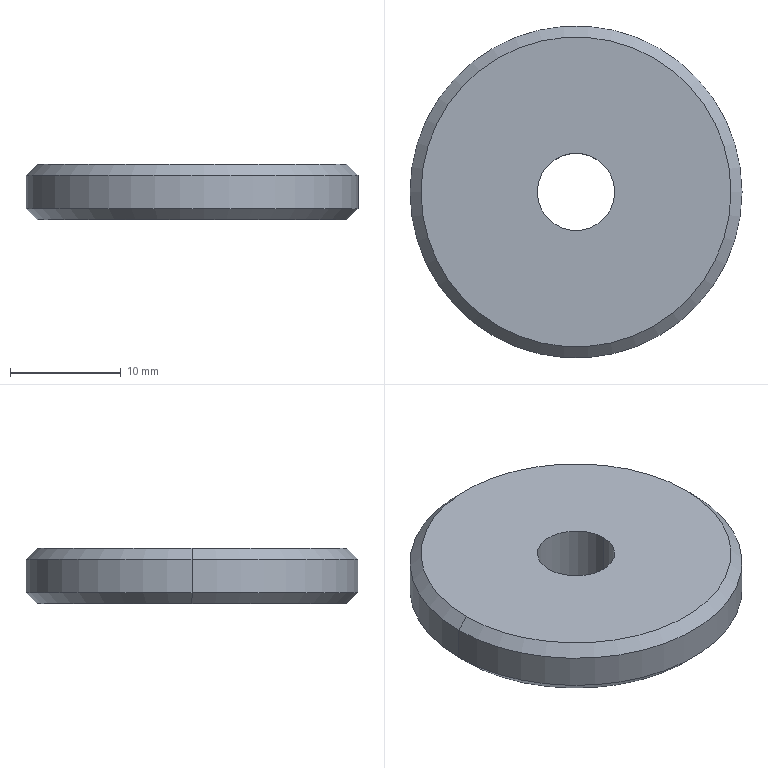Part | STEP file | TJ-DHQM-003-015 | 1 solid | 10 faces | box 30 x 30 x 5 mm | volume 3250 mm3 | cone 4 | cylinder 4 | plane 2 | commonest cylinder face diameters 7 x2 30 x2
STEP:
#1=CARTESIAN_POINT('',(14.,0.,5.));
#2=VERTEX_POINT('',#1);
#3=CARTESIAN_POINT('',(-14.,0.,5.));
#4=VERTEX_POINT('',#3);
#5=CARTESIAN_POINT('',(0.,0.,5.));
#6=DIRECTION('',(0.,0.,1.));
#7=DIRECTION('',(1.,0.,0.));
#8=AXIS2_PLACEMENT_3D('',#5,#6,#7);
#9=CIRCLE('',#8,14.);
#10=EDGE_CURVE('',#2,#4,#9,.T.);
#11=ORIENTED_EDGE('',*,*,#10,.F.);
#12=CARTESIAN_POINT('',(15.,0.,4.));
#13=VERTEX_POINT('',#12);
#14=CARTESIAN_POINT('',(14.,0.,5.));
#15=DIRECTION('',(0.7071,0.,-0.7071));
#16=VECTOR('',#15,1000.);
#17=LINE('',#14,#16);
#18=EDGE_CURVE('',#2,#13,#17,.T.);
#19=ORIENTED_EDGE('',*,*,#18,.T.);
#20=CARTESIAN_POINT('',(-15.,0.,4.));
#21=VERTEX_POINT('',#20);
#22=CARTESIAN_POINT('',(0.,0.,4.));
#23=DIRECTION('',(0.,0.,-1.));
#24=DIRECTION('',(1.,0.,0.));
#25=AXIS2_PLACEMENT_3D('',#22,#23,#24);
#26=CIRCLE('',#25,15.);
#27=EDGE_CURVE('',#21,#13,#26,.T.);
#28=ORIENTED_EDGE('',*,*,#27,.F.);
#29=CARTESIAN_POINT('',(-14.,0.,5.));
#30=DIRECTION('',(-0.7071,0.,-0.7071));
#31=VECTOR('',#30,1000.);
#32=LINE('',#29,#31);
#33=EDGE_CURVE('',#4,#21,#32,.T.);
#34=ORIENTED_EDGE('',*,*,#33,.F.);
#35=EDGE_LOOP('',(#11,#19,#28,#34));
#36=FACE_OUTER_BOUND('',#35,.T.);
#37=CARTESIAN_POINT('',(0.,0.,5.));
#38=DIRECTION('',(0.,0.,-1.));
#39=DIRECTION('',(-1.,0.,0.));
#40=AXIS2_PLACEMENT_3D('',#37,#38,#39);
#41=CONICAL_SURFACE('',#40,14.,0.7854);
#42=ADVANCED_FACE('',(#36),#41,.T.);
#43=CARTESIAN_POINT('',(-14.,0.,0.));
#44=VERTEX_POINT('',#43);
#45=CARTESIAN_POINT('',(14.,0.,0.));
#46=VERTEX_POINT('',#45);
#47=CARTESIAN_POINT('',(0.,0.,0.));
#48=DIRECTION('',(0.,0.,-1.));
#49=DIRECTION('',(1.,0.,0.));
#50=AXIS2_PLACEMENT_3D('',#47,#48,#49);
#51=CIRCLE('',#50,14.);
#52=EDGE_CURVE('',#44,#46,#51,.T.);
#53=ORIENTED_EDGE('',*,*,#52,.F.);
#54=CARTESIAN_POINT('',(-15.,0.,1.));
#55=VERTEX_POINT('',#54);
#56=CARTESIAN_POINT('',(-15.,0.,1.));
#57=DIRECTION('',(-0.7071,0.,0.7071));
#58=VECTOR('',#57,1000.);
#59=LINE('',#56,#58);
#60=EDGE_CURVE('',#44,#55,#59,.T.);
#61=ORIENTED_EDGE('',*,*,#60,.T.);
#62=CARTESIAN_POINT('',(15.,0.,1.));
#63=VERTEX_POINT('',#62);
#64=CARTESIAN_POINT('',(0.,0.,1.));
#65=DIRECTION('',(0.,0.,1.));
#66=DIRECTION('',(1.,0.,0.));
#67=AXIS2_PLACEMENT_3D('',#64,#65,#66);
#68=CIRCLE('',#67,15.);
#69=EDGE_CURVE('',#63,#55,#68,.T.);
#70=ORIENTED_EDGE('',*,*,#69,.F.);
#71=CARTESIAN_POINT('',(15.,0.,1.));
#72=DIRECTION('',(0.7071,0.,0.7071));
#73=VECTOR('',#72,1000.);
#74=LINE('',#71,#73);
#75=EDGE_CURVE('',#46,#63,#74,.T.);
#76=ORIENTED_EDGE('',*,*,#75,.F.);
#77=EDGE_LOOP('',(#53,#61,#70,#76));
#78=FACE_OUTER_BOUND('',#77,.T.);
#79=CARTESIAN_POINT('',(0.,0.,1.));
#80=DIRECTION('',(0.,0.,1.));
#81=DIRECTION('',(1.,0.,0.));
#82=AXIS2_PLACEMENT_3D('',#79,#80,#81);
#83=CONICAL_SURFACE('',#82,15.,0.7854);
#84=ADVANCED_FACE('',(#78),#83,.T.);
#85=CARTESIAN_POINT('',(-3.5,0.,0.));
#86=VERTEX_POINT('',#85);
#87=CARTESIAN_POINT('',(3.5,0.,0.));
#88=VERTEX_POINT('',#87);
#89=CARTESIAN_POINT('',(0.,0.,0.));
#90=DIRECTION('',(0.,0.,1.));
#91=DIRECTION('',(1.,0.,0.));
#92=AXIS2_PLACEMENT_3D('',#89,#90,#91);
#93=CIRCLE('',#92,3.5);
#94=EDGE_CURVE('',#86,#88,#93,.T.);
#95=ORIENTED_EDGE('',*,*,#94,.F.);
#96=CARTESIAN_POINT('',(-3.5,0.,5.));
#97=VERTEX_POINT('',#96);
#98=CARTESIAN_POINT('',(-3.5,0.,0.));
#99=DIRECTION('',(0.,0.,1.));
#100=VECTOR('',#99,1000.);
#101=LINE('',#98,#100);
#102=EDGE_CURVE('',#86,#97,#101,.T.);
#103=ORIENTED_EDGE('',*,*,#102,.T.);
#104=CARTESIAN_POINT('',(3.5,0.,5.));
#105=VERTEX_POINT('',#104);
#106=CARTESIAN_POINT('',(0.,0.,5.));
#107=DIRECTION('',(0.,0.,1.));
#108=DIRECTION('',(1.,0.,0.));
#109=AXIS2_PLACEMENT_3D('',#106,#107,#108);
#110=CIRCLE('',#109,3.5);
#111=EDGE_CURVE('',#97,#105,#110,.T.);
#112=ORIENTED_EDGE('',*,*,#111,.T.);
#113=CARTESIAN_POINT('',(3.5,0.,0.));
#114=DIRECTION('',(0.,0.,1.));
#115=VECTOR('',#114,1000.);
#116=LINE('',#113,#115);
#117=EDGE_CURVE('',#88,#105,#116,.T.);
#118=ORIENTED_EDGE('',*,*,#117,.F.);
#119=EDGE_LOOP('',(#95,#103,#112,#118));
#120=FACE_OUTER_BOUND('',#119,.T.);
#121=CARTESIAN_POINT('',(0.,0.,0.));
#122=DIRECTION('',(0.,0.,1.));
#123=DIRECTION('',(1.,0.,0.));
#124=AXIS2_PLACEMENT_3D('',#121,#122,#123);
#125=CYLINDRICAL_SURFACE('',#124,3.5);
#126=ADVANCED_FACE('',(#120),#125,.F.);
#127=ORIENTED_EDGE('',*,*,#27,.T.);
#128=CARTESIAN_POINT('',(15.,0.,5.));
#129=DIRECTION('',(0.,0.,-1.));
#130=VECTOR('',#129,1000.);
#131=LINE('',#128,#130);
#132=EDGE_CURVE('',#13,#63,#131,.T.);
#133=ORIENTED_EDGE('',*,*,#132,.T.);
#134=ORIENTED_EDGE('',*,*,#69,.T.);
#135=CARTESIAN_POINT('',(-15.,0.,5.));
#136=DIRECTION('',(0.,0.,-1.));
#137=VECTOR('',#136,1000.);
#138=LINE('',#135,#137);
#139=EDGE_CURVE('',#21,#55,#138,.T.);
#140=ORIENTED_EDGE('',*,*,#139,.F.);
#141=EDGE_LOOP('',(#127,#133,#134,#140));
#142=FACE_OUTER_BOUND('',#141,.T.);
#143=CARTESIAN_POINT('',(0.,0.,5.));
#144=DIRECTION('',(0.,0.,-1.));
#145=DIRECTION('',(-1.,0.,0.));
#146=AXIS2_PLACEMENT_3D('',#143,#144,#145);
#147=CYLINDRICAL_SURFACE('',#146,15.);
#148=ADVANCED_FACE('',(#142),#147,.T.);
#149=ORIENTED_EDGE('',*,*,#132,.F.);
#150=CARTESIAN_POINT('',(0.,0.,4.));
#151=DIRECTION('',(0.,0.,-1.));
#152=DIRECTION('',(1.,0.,0.));
#153=AXIS2_PLACEMENT_3D('',#150,#151,#152);
#154=CIRCLE('',#153,15.);
#155=EDGE_CURVE('',#13,#21,#154,.T.);
#156=ORIENTED_EDGE('',*,*,#155,.T.);
#157=ORIENTED_EDGE('',*,*,#139,.T.);
#158=CARTESIAN_POINT('',(0.,0.,1.));
#159=DIRECTION('',(0.,0.,1.));
#160=DIRECTION('',(1.,0.,0.));
#161=AXIS2_PLACEMENT_3D('',#158,#159,#160);
#162=CIRCLE('',#161,15.);
#163=EDGE_CURVE('',#55,#63,#162,.T.);
#164=ORIENTED_EDGE('',*,*,#163,.T.);
#165=EDGE_LOOP('',(#149,#156,#157,#164));
#166=FACE_OUTER_BOUND('',#165,.T.);
#167=CARTESIAN_POINT('',(0.,0.,5.));
#168=DIRECTION('',(0.,0.,-1.));
#169=DIRECTION('',(-1.,0.,0.));
#170=AXIS2_PLACEMENT_3D('',#167,#168,#169);
#171=CYLINDRICAL_SURFACE('',#170,15.);
#172=ADVANCED_FACE('',(#166),#171,.T.);
#173=CARTESIAN_POINT('',(0.,0.,5.));
#174=DIRECTION('',(0.,0.,1.));
#175=DIRECTION('',(1.,0.,0.));
#176=AXIS2_PLACEMENT_3D('',#173,#174,#175);
#177=CIRCLE('',#176,14.);
#178=EDGE_CURVE('',#4,#2,#177,.T.);
#179=ORIENTED_EDGE('',*,*,#178,.T.);
#180=ORIENTED_EDGE('',*,*,#10,.T.);
#181=EDGE_LOOP('',(#179,#180));
#182=FACE_OUTER_BOUND('',#181,.T.);
#183=CARTESIAN_POINT('',(0.,0.,5.));
#184=DIRECTION('',(0.,0.,1.));
#185=DIRECTION('',(1.,0.,0.));
#186=AXIS2_PLACEMENT_3D('',#183,#184,#185);
#187=CIRCLE('',#186,3.5);
#188=EDGE_CURVE('',#105,#97,#187,.T.);
#189=ORIENTED_EDGE('',*,*,#188,.F.);
#190=ORIENTED_EDGE('',*,*,#111,.F.);
#191=EDGE_LOOP('',(#189,#190));
#192=FACE_BOUND('',#191,.T.);
#193=CARTESIAN_POINT('',(0.,0.,5.));
#194=DIRECTION('',(0.,0.,1.));
#195=DIRECTION('',(1.,0.,0.));
#196=AXIS2_PLACEMENT_3D('',#193,#194,#195);
#197=PLANE('',#196);
#198=ADVANCED_FACE('',(#182,#192),#197,.T.);
#199=CARTESIAN_POINT('',(0.,0.,0.));
#200=DIRECTION('',(0.,0.,-1.));
#201=DIRECTION('',(1.,0.,0.));
#202=AXIS2_PLACEMENT_3D('',#199,#200,#201);
#203=CIRCLE('',#202,14.);
#204=EDGE_CURVE('',#46,#44,#203,.T.);
#205=ORIENTED_EDGE('',*,*,#204,.T.);
#206=ORIENTED_EDGE('',*,*,#52,.T.);
#207=EDGE_LOOP('',(#205,#206));
#208=FACE_OUTER_BOUND('',#207,.T.);
#209=CARTESIAN_POINT('',(0.,0.,0.));
#210=DIRECTION('',(0.,0.,1.));
#211=DIRECTION('',(1.,0.,0.));
#212=AXIS2_PLACEMENT_3D('',#209,#210,#211);
#213=CIRCLE('',#212,3.5);
#214=EDGE_CURVE('',#88,#86,#213,.T.);
#215=ORIENTED_EDGE('',*,*,#214,.T.);
#216=ORIENTED_EDGE('',*,*,#94,.T.);
#217=EDGE_LOOP('',(#215,#216));
#218=FACE_BOUND('',#217,.T.);
#219=CARTESIAN_POINT('',(0.,0.,0.));
#220=DIRECTION('',(0.,0.,1.));
#221=DIRECTION('',(1.,0.,0.));
#222=AXIS2_PLACEMENT_3D('',#219,#220,#221);
#223=PLANE('',#222);
#224=ADVANCED_FACE('',(#208,#218),#223,.F.);
#225=ORIENTED_EDGE('',*,*,#102,.F.);
#226=ORIENTED_EDGE('',*,*,#214,.F.);
#227=ORIENTED_EDGE('',*,*,#117,.T.);
#228=ORIENTED_EDGE('',*,*,#188,.T.);
#229=EDGE_LOOP('',(#225,#226,#227,#228));
#230=FACE_OUTER_BOUND('',#229,.T.);
#231=CARTESIAN_POINT('',(0.,0.,0.));
#232=DIRECTION('',(0.,0.,1.));
#233=DIRECTION('',(1.,0.,0.));
#234=AXIS2_PLACEMENT_3D('',#231,#232,#233);
#235=CYLINDRICAL_SURFACE('',#234,3.5);
#236=ADVANCED_FACE('',(#230),#235,.F.);
#237=ORIENTED_EDGE('',*,*,#60,.F.);
#238=ORIENTED_EDGE('',*,*,#204,.F.);
#239=ORIENTED_EDGE('',*,*,#75,.T.);
#240=ORIENTED_EDGE('',*,*,#163,.F.);
#241=EDGE_LOOP('',(#237,#238,#239,#240));
#242=FACE_OUTER_BOUND('',#241,.T.);
#243=CARTESIAN_POINT('',(0.,0.,1.));
#244=DIRECTION('',(0.,0.,1.));
#245=DIRECTION('',(1.,0.,0.));
#246=AXIS2_PLACEMENT_3D('',#243,#244,#245);
#247=CONICAL_SURFACE('',#246,15.,0.7854);
#248=ADVANCED_FACE('',(#242),#247,.T.);
#249=ORIENTED_EDGE('',*,*,#18,.F.);
#250=ORIENTED_EDGE('',*,*,#178,.F.);
#251=ORIENTED_EDGE('',*,*,#33,.T.);
#252=ORIENTED_EDGE('',*,*,#155,.F.);
#253=EDGE_LOOP('',(#249,#250,#251,#252));
#254=FACE_OUTER_BOUND('',#253,.T.);
#255=CARTESIAN_POINT('',(0.,0.,5.));
#256=DIRECTION('',(0.,0.,-1.));
#257=DIRECTION('',(-1.,0.,0.));
#258=AXIS2_PLACEMENT_3D('',#255,#256,#257);
#259=CONICAL_SURFACE('',#258,14.,0.7854);
#260=ADVANCED_FACE('',(#254),#259,.T.);
#261=CLOSED_SHELL('',(#42,#84,#126,#148,#172,#198,#224,#236,#248,#260));
#262=MANIFOLD_SOLID_BREP('',#261);
#263=CARTESIAN_POINT('',(0.,0.,0.));
#264=DIRECTION('',(0.,0.,1.));
#265=DIRECTION('',(1.,0.,0.));
#266=AXIS2_PLACEMENT_3D('',#263,#264,#265);
#267=(LENGTH_UNIT()NAMED_UNIT(*)SI_UNIT(.MILLI.,.METRE.));
#268=UNCERTAINTY_MEASURE_WITH_UNIT(LENGTH_MEASURE(0.00001),#267,'','');
#269=(NAMED_UNIT(*)PLANE_ANGLE_UNIT()SI_UNIT($,.RADIAN.));
#270=(NAMED_UNIT(*)SI_UNIT($,.STERADIAN.)SOLID_ANGLE_UNIT());
#271=(GEOMETRIC_REPRESENTATION_CONTEXT(3)GLOBAL_UNCERTAINTY_ASSIGNED_CONTEXT((#268))GLOBAL_UNIT_ASSIGNED_CONTEXT((#267,#269,#270))REPRESENTATION_CONTEXT('',''));
#272=ADVANCED_BREP_SHAPE_REPRESENTATION('',(#262,#266),#271);